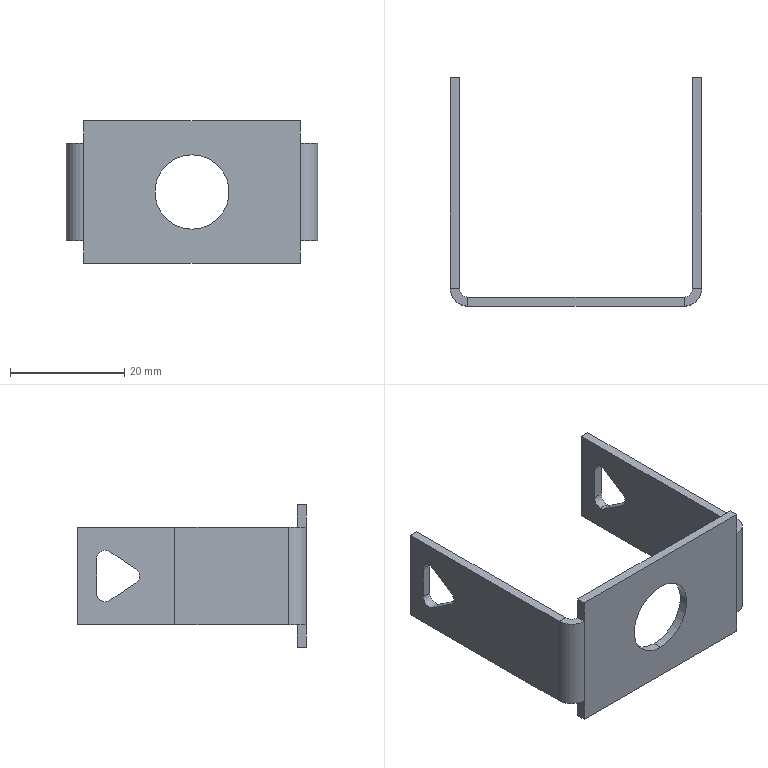Part | SolidWorks | features ICE 6, FlatPattern 1, MirrorPattern 1, SMBaseFlange 1, SheetMetal 1 | 1 solid | 48 faces | box 44 x 40 x 25 mm | volume 3354 mm3 | plane 34 | cylinder 14 | commonest cylinder face diameters 3 x10 6.2 x2 13 x2
STEP:
#1=CARTESIAN_POINT('',(42.401,35.2,-4.497));
#2=VERTEX_POINT('',#1);
#3=CARTESIAN_POINT('',(42.401,36.7,-2.997));
#4=VERTEX_POINT('',#3);
#5=CARTESIAN_POINT('',(42.401,35.2,-2.997));
#6=DIRECTION('',(1.,0.,0.));
#7=DIRECTION('',(0.,0.,-1.));
#8=AXIS2_PLACEMENT_3D('',#5,#6,#7);
#9=CIRCLE('',#8,1.5);
#10=EDGE_CURVE('',#2,#4,#9,.T.);
#11=ORIENTED_EDGE('',*,*,#10,.F.);
#12=CARTESIAN_POINT('',(43.999,35.2,-4.497));
#13=VERTEX_POINT('',#12);
#14=CARTESIAN_POINT('',(40.9,35.2,-4.497));
#15=DIRECTION('',(1.,0.,0.));
#16=VECTOR('',#15,1000.);
#17=LINE('',#14,#16);
#18=EDGE_CURVE('',#2,#13,#17,.T.);
#19=ORIENTED_EDGE('',*,*,#18,.T.);
#20=CARTESIAN_POINT('',(43.999,36.7,-2.997));
#21=VERTEX_POINT('',#20);
#22=CARTESIAN_POINT('',(43.999,35.2,-2.997));
#23=DIRECTION('',(-1.,0.,0.));
#24=DIRECTION('',(0.,0.,1.));
#25=AXIS2_PLACEMENT_3D('',#22,#23,#24);
#26=CIRCLE('',#25,1.5);
#27=EDGE_CURVE('',#21,#13,#26,.T.);
#28=ORIENTED_EDGE('',*,*,#27,.F.);
#29=CARTESIAN_POINT('',(40.9,36.7,-2.997));
#30=DIRECTION('',(1.,0.,0.));
#31=VECTOR('',#30,1000.);
#32=LINE('',#29,#31);
#33=EDGE_CURVE('',#4,#21,#32,.T.);
#34=ORIENTED_EDGE('',*,*,#33,.F.);
#35=EDGE_LOOP('',(#11,#19,#28,#34));
#36=FACE_OUTER_BOUND('',#35,.T.);
#37=CARTESIAN_POINT('',(40.9,35.2,-2.997));
#38=DIRECTION('',(1.,0.,0.));
#39=DIRECTION('',(0.,0.,-1.));
#40=AXIS2_PLACEMENT_3D('',#37,#38,#39);
#41=CYLINDRICAL_SURFACE('',#40,1.5);
#42=ADVANCED_FACE('',(#36),#41,.F.);
#43=CARTESIAN_POINT('',(22.,0.,-6.5));
#44=VERTEX_POINT('',#43);
#45=CARTESIAN_POINT('',(22.,0.,6.5));
#46=VERTEX_POINT('',#45);
#47=CARTESIAN_POINT('',(22.,0.,0.));
#48=DIRECTION('',(0.,1.,0.));
#49=DIRECTION('',(0.,0.,-1.));
#50=AXIS2_PLACEMENT_3D('',#47,#48,#49);
#51=CIRCLE('',#50,6.5);
#52=EDGE_CURVE('',#44,#46,#51,.T.);
#53=ORIENTED_EDGE('',*,*,#52,.F.);
#54=CARTESIAN_POINT('',(22.,1.6,-6.5));
#55=VERTEX_POINT('',#54);
#56=CARTESIAN_POINT('',(22.,-0.001,-6.5));
#57=DIRECTION('',(0.,1.,0.));
#58=VECTOR('',#57,1000.);
#59=LINE('',#56,#58);
#60=EDGE_CURVE('',#44,#55,#59,.T.);
#61=ORIENTED_EDGE('',*,*,#60,.T.);
#62=CARTESIAN_POINT('',(22.,1.6,6.5));
#63=VERTEX_POINT('',#62);
#64=CARTESIAN_POINT('',(22.,1.6,0.));
#65=DIRECTION('',(0.,1.,0.));
#66=DIRECTION('',(0.,0.,1.));
#67=AXIS2_PLACEMENT_3D('',#64,#65,#66);
#68=CIRCLE('',#67,6.5);
#69=EDGE_CURVE('',#55,#63,#68,.T.);
#70=ORIENTED_EDGE('',*,*,#69,.T.);
#71=CARTESIAN_POINT('',(22.,-0.001,6.5));
#72=DIRECTION('',(0.,1.,0.));
#73=VECTOR('',#72,1000.);
#74=LINE('',#71,#73);
#75=EDGE_CURVE('',#46,#63,#74,.T.);
#76=ORIENTED_EDGE('',*,*,#75,.F.);
#77=EDGE_LOOP('',(#53,#61,#70,#76));
#78=FACE_OUTER_BOUND('',#77,.T.);
#79=CARTESIAN_POINT('',(22.,-0.001,0.));
#80=DIRECTION('',(0.,1.,0.));
#81=DIRECTION('',(0.,0.,1.));
#82=AXIS2_PLACEMENT_3D('',#79,#80,#81);
#83=CYLINDRICAL_SURFACE('',#82,6.5);
#84=ADVANCED_FACE('',(#78),#83,.F.);
#85=CARTESIAN_POINT('',(1.599,35.2,4.497));
#86=VERTEX_POINT('',#85);
#87=CARTESIAN_POINT('',(1.599,36.7,2.997));
#88=VERTEX_POINT('',#87);
#89=CARTESIAN_POINT('',(1.599,35.2,2.997));
#90=DIRECTION('',(-1.,0.,0.));
#91=DIRECTION('',(0.,0.,-1.));
#92=AXIS2_PLACEMENT_3D('',#89,#90,#91);
#93=CIRCLE('',#92,1.5);
#94=EDGE_CURVE('',#86,#88,#93,.T.);
#95=ORIENTED_EDGE('',*,*,#94,.F.);
#96=CARTESIAN_POINT('',(0.01,35.2,4.497));
#97=VERTEX_POINT('',#96);
#98=CARTESIAN_POINT('',(3.1,35.2,4.497));
#99=DIRECTION('',(-1.,0.,0.));
#100=VECTOR('',#99,1000.);
#101=LINE('',#98,#100);
#102=EDGE_CURVE('',#86,#97,#101,.T.);
#103=ORIENTED_EDGE('',*,*,#102,.T.);
#104=CARTESIAN_POINT('',(0.01,36.7,2.997));
#105=VERTEX_POINT('',#104);
#106=CARTESIAN_POINT('',(0.01,35.2,2.997));
#107=DIRECTION('',(1.,0.,0.));
#108=DIRECTION('',(0.,0.,1.));
#109=AXIS2_PLACEMENT_3D('',#106,#107,#108);
#110=CIRCLE('',#109,1.5);
#111=EDGE_CURVE('',#105,#97,#110,.T.);
#112=ORIENTED_EDGE('',*,*,#111,.F.);
#113=CARTESIAN_POINT('',(3.1,36.7,2.997));
#114=DIRECTION('',(-1.,0.,0.));
#115=VECTOR('',#114,1000.);
#116=LINE('',#113,#115);
#117=EDGE_CURVE('',#88,#105,#116,.T.);
#118=ORIENTED_EDGE('',*,*,#117,.F.);
#119=EDGE_LOOP('',(#95,#103,#112,#118));
#120=FACE_OUTER_BOUND('',#119,.T.);
#121=CARTESIAN_POINT('',(3.1,35.2,2.997));
#122=DIRECTION('',(-1.,0.,0.));
#123=DIRECTION('',(0.,0.,1.));
#124=AXIS2_PLACEMENT_3D('',#121,#122,#123);
#125=CYLINDRICAL_SURFACE('',#124,1.5);
#126=ADVANCED_FACE('',(#120),#125,.F.);
#127=CARTESIAN_POINT('',(1.599,40.,8.5));
#128=VERTEX_POINT('',#127);
#129=CARTESIAN_POINT('',(0.01,40.,8.5));
#130=VERTEX_POINT('',#129);
#131=CARTESIAN_POINT('',(3.1,40.,8.5));
#132=DIRECTION('',(-1.,0.,0.));
#133=VECTOR('',#132,1000.);
#134=LINE('',#131,#133);
#135=EDGE_CURVE('',#128,#130,#134,.T.);
#136=ORIENTED_EDGE('',*,*,#135,.F.);
#137=CARTESIAN_POINT('',(1.599,40.,-8.5));
#138=VERTEX_POINT('',#137);
#139=CARTESIAN_POINT('',(1.599,40.,8.5));
#140=DIRECTION('',(0.,0.,1.));
#141=VECTOR('',#140,1000.);
#142=LINE('',#139,#141);
#143=EDGE_CURVE('',#138,#128,#142,.T.);
#144=ORIENTED_EDGE('',*,*,#143,.F.);
#145=CARTESIAN_POINT('',(0.01,40.,-8.5));
#146=VERTEX_POINT('',#145);
#147=CARTESIAN_POINT('',(3.1,40.,-8.5));
#148=DIRECTION('',(-1.,0.,0.));
#149=VECTOR('',#148,1000.);
#150=LINE('',#147,#149);
#151=EDGE_CURVE('',#138,#146,#150,.T.);
#152=ORIENTED_EDGE('',*,*,#151,.T.);
#153=CARTESIAN_POINT('',(0.01,40.,-8.5));
#154=DIRECTION('',(0.,0.,-1.));
#155=VECTOR('',#154,1000.);
#156=LINE('',#153,#155);
#157=EDGE_CURVE('',#130,#146,#156,.T.);
#158=ORIENTED_EDGE('',*,*,#157,.F.);
#159=EDGE_LOOP('',(#136,#144,#152,#158));
#160=FACE_OUTER_BOUND('',#159,.T.);
#161=CARTESIAN_POINT('',(0.,40.,12.5));
#162=DIRECTION('',(0.,1.,0.));
#163=DIRECTION('',(0.,0.,1.));
#164=AXIS2_PLACEMENT_3D('',#161,#162,#163);
#165=PLANE('',#164);
#166=ADVANCED_FACE('',(#160),#165,.T.);
#167=CARTESIAN_POINT('',(1.599,29.872,-1.248));
#168=VERTEX_POINT('',#167);
#169=CARTESIAN_POINT('',(1.599,29.872,1.248));
#170=VERTEX_POINT('',#169);
#171=CARTESIAN_POINT('',(1.599,30.704,0.));
#172=DIRECTION('',(-1.,0.,0.));
#173=DIRECTION('',(0.,0.,-1.));
#174=AXIS2_PLACEMENT_3D('',#171,#172,#173);
#175=CIRCLE('',#174,1.5);
#176=EDGE_CURVE('',#168,#170,#175,.T.);
#177=ORIENTED_EDGE('',*,*,#176,.F.);
#178=CARTESIAN_POINT('',(0.01,29.872,-1.248));
#179=VERTEX_POINT('',#178);
#180=CARTESIAN_POINT('',(3.1,29.872,-1.248));
#181=DIRECTION('',(-1.,0.,0.));
#182=VECTOR('',#181,1000.);
#183=LINE('',#180,#182);
#184=EDGE_CURVE('',#168,#179,#183,.T.);
#185=ORIENTED_EDGE('',*,*,#184,.T.);
#186=CARTESIAN_POINT('',(0.01,29.872,1.248));
#187=VERTEX_POINT('',#186);
#188=CARTESIAN_POINT('',(0.01,30.704,0.));
#189=DIRECTION('',(1.,0.,0.));
#190=DIRECTION('',(0.,0.,1.));
#191=AXIS2_PLACEMENT_3D('',#188,#189,#190);
#192=CIRCLE('',#191,1.5);
#193=EDGE_CURVE('',#187,#179,#192,.T.);
#194=ORIENTED_EDGE('',*,*,#193,.F.);
#195=CARTESIAN_POINT('',(3.1,29.872,1.248));
#196=DIRECTION('',(-1.,0.,0.));
#197=VECTOR('',#196,1000.);
#198=LINE('',#195,#197);
#199=EDGE_CURVE('',#170,#187,#198,.T.);
#200=ORIENTED_EDGE('',*,*,#199,.F.);
#201=EDGE_LOOP('',(#177,#185,#194,#200));
#202=FACE_OUTER_BOUND('',#201,.T.);
#203=CARTESIAN_POINT('',(3.1,30.704,0.));
#204=DIRECTION('',(-1.,0.,0.));
#205=DIRECTION('',(0.,0.,1.));
#206=AXIS2_PLACEMENT_3D('',#203,#204,#205);
#207=CYLINDRICAL_SURFACE('',#206,1.5);
#208=ADVANCED_FACE('',(#202),#207,.F.);
#209=CARTESIAN_POINT('',(1.599,34.368,-4.245));
#210=VERTEX_POINT('',#209);
#211=CARTESIAN_POINT('',(1.599,29.872,-1.248));
#212=DIRECTION('',(0.,-0.8321,0.5547));
#213=VECTOR('',#212,1000.);
#214=LINE('',#211,#213);
#215=EDGE_CURVE('',#210,#168,#214,.T.);
#216=ORIENTED_EDGE('',*,*,#215,.F.);
#217=CARTESIAN_POINT('',(0.01,34.368,-4.245));
#218=VERTEX_POINT('',#217);
#219=CARTESIAN_POINT('',(3.1,34.368,-4.245));
#220=DIRECTION('',(-1.,0.,0.));
#221=VECTOR('',#220,1000.);
#222=LINE('',#219,#221);
#223=EDGE_CURVE('',#210,#218,#222,.T.);
#224=ORIENTED_EDGE('',*,*,#223,.T.);
#225=CARTESIAN_POINT('',(0.01,29.872,-1.248));
#226=DIRECTION('',(0.,0.8321,-0.5547));
#227=VECTOR('',#226,1000.);
#228=LINE('',#225,#227);
#229=EDGE_CURVE('',#179,#218,#228,.T.);
#230=ORIENTED_EDGE('',*,*,#229,.F.);
#231=ORIENTED_EDGE('',*,*,#184,.F.);
#232=EDGE_LOOP('',(#216,#224,#230,#231));
#233=FACE_OUTER_BOUND('',#232,.T.);
#234=CARTESIAN_POINT('',(3.1,29.872,-1.248));
#235=DIRECTION('',(0.,-0.5547,-0.8321));
#236=DIRECTION('',(0.,0.8321,-0.5547));
#237=AXIS2_PLACEMENT_3D('',#234,#235,#236);
#238=PLANE('',#237);
#239=ADVANCED_FACE('',(#233),#238,.F.);
#240=CARTESIAN_POINT('',(1.599,36.7,-2.997));
#241=VERTEX_POINT('',#240);
#242=CARTESIAN_POINT('',(1.599,35.2,-2.997));
#243=DIRECTION('',(-1.,0.,0.));
#244=DIRECTION('',(0.,0.,-1.));
#245=AXIS2_PLACEMENT_3D('',#242,#243,#244);
#246=CIRCLE('',#245,1.5);
#247=EDGE_CURVE('',#241,#210,#246,.T.);
#248=ORIENTED_EDGE('',*,*,#247,.F.);
#249=CARTESIAN_POINT('',(0.01,36.7,-2.997));
#250=VERTEX_POINT('',#249);
#251=CARTESIAN_POINT('',(3.1,36.7,-2.997));
#252=DIRECTION('',(-1.,0.,0.));
#253=VECTOR('',#252,1000.);
#254=LINE('',#251,#253);
#255=EDGE_CURVE('',#241,#250,#254,.T.);
#256=ORIENTED_EDGE('',*,*,#255,.T.);
#257=CARTESIAN_POINT('',(0.01,35.2,-2.997));
#258=DIRECTION('',(1.,0.,0.));
#259=DIRECTION('',(0.,0.,1.));
#260=AXIS2_PLACEMENT_3D('',#257,#258,#259);
#261=CIRCLE('',#260,1.5);
#262=EDGE_CURVE('',#218,#250,#261,.T.);
#263=ORIENTED_EDGE('',*,*,#262,.F.);
#264=ORIENTED_EDGE('',*,*,#223,.F.);
#265=EDGE_LOOP('',(#248,#256,#263,#264));
#266=FACE_OUTER_BOUND('',#265,.T.);
#267=CARTESIAN_POINT('',(3.1,35.2,-2.997));
#268=DIRECTION('',(-1.,0.,0.));
#269=DIRECTION('',(0.,0.,1.));
#270=AXIS2_PLACEMENT_3D('',#267,#268,#269);
#271=CYLINDRICAL_SURFACE('',#270,1.5);
#272=ADVANCED_FACE('',(#266),#271,.F.);
#273=CARTESIAN_POINT('',(1.599,36.7,-2.997));
#274=DIRECTION('',(0.,0.,-1.));
#275=VECTOR('',#274,1000.);
#276=LINE('',#273,#275);
#277=EDGE_CURVE('',#88,#241,#276,.T.);
#278=ORIENTED_EDGE('',*,*,#277,.F.);
#279=ORIENTED_EDGE('',*,*,#117,.T.);
#280=CARTESIAN_POINT('',(0.01,36.7,-2.997));
#281=DIRECTION('',(0.,0.,1.));
#282=VECTOR('',#281,1000.);
#283=LINE('',#280,#282);
#284=EDGE_CURVE('',#250,#105,#283,.T.);
#285=ORIENTED_EDGE('',*,*,#284,.F.);
#286=ORIENTED_EDGE('',*,*,#255,.F.);
#287=EDGE_LOOP('',(#278,#279,#285,#286));
#288=FACE_OUTER_BOUND('',#287,.T.);
#289=CARTESIAN_POINT('',(3.1,36.7,-2.997));
#290=DIRECTION('',(0.,1.,0.));
#291=DIRECTION('',(0.,0.,1.));
#292=AXIS2_PLACEMENT_3D('',#289,#290,#291);
#293=PLANE('',#292);
#294=ADVANCED_FACE('',(#288),#293,.F.);
#295=ORIENTED_EDGE('',*,*,#102,.F.);
#296=CARTESIAN_POINT('',(1.599,34.368,4.245));
#297=VERTEX_POINT('',#296);
#298=CARTESIAN_POINT('',(1.599,35.2,2.997));
#299=DIRECTION('',(-1.,0.,0.));
#300=DIRECTION('',(0.,0.,-1.));
#301=AXIS2_PLACEMENT_3D('',#298,#299,#300);
#302=CIRCLE('',#301,1.5);
#303=EDGE_CURVE('',#297,#86,#302,.T.);
#304=ORIENTED_EDGE('',*,*,#303,.F.);
#305=CARTESIAN_POINT('',(0.01,34.368,4.245));
#306=VERTEX_POINT('',#305);
#307=CARTESIAN_POINT('',(3.1,34.368,4.245));
#308=DIRECTION('',(-1.,0.,0.));
#309=VECTOR('',#308,1000.);
#310=LINE('',#307,#309);
#311=EDGE_CURVE('',#297,#306,#310,.T.);
#312=ORIENTED_EDGE('',*,*,#311,.T.);
#313=CARTESIAN_POINT('',(0.01,35.2,2.997));
#314=DIRECTION('',(1.,0.,0.));
#315=DIRECTION('',(0.,0.,1.));
#316=AXIS2_PLACEMENT_3D('',#313,#314,#315);
#317=CIRCLE('',#316,1.5);
#318=EDGE_CURVE('',#97,#306,#317,.T.);
#319=ORIENTED_EDGE('',*,*,#318,.F.);
#320=EDGE_LOOP('',(#295,#304,#312,#319));
#321=FACE_OUTER_BOUND('',#320,.T.);
#322=CARTESIAN_POINT('',(3.1,35.2,2.997));
#323=DIRECTION('',(-1.,0.,0.));
#324=DIRECTION('',(0.,0.,1.));
#325=AXIS2_PLACEMENT_3D('',#322,#323,#324);
#326=CYLINDRICAL_SURFACE('',#325,1.5);
#327=ADVANCED_FACE('',(#321),#326,.F.);
#328=CARTESIAN_POINT('',(1.599,29.872,1.248));
#329=DIRECTION('',(0.,0.8321,0.5547));
#330=VECTOR('',#329,1000.);
#331=LINE('',#328,#330);
#332=EDGE_CURVE('',#170,#297,#331,.T.);
#333=ORIENTED_EDGE('',*,*,#332,.F.);
#334=ORIENTED_EDGE('',*,*,#199,.T.);
#335=CARTESIAN_POINT('',(0.01,29.872,1.248));
#336=DIRECTION('',(0.,-0.8321,-0.5547));
#337=VECTOR('',#336,1000.);
#338=LINE('',#335,#337);
#339=EDGE_CURVE('',#306,#187,#338,.T.);
#340=ORIENTED_EDGE('',*,*,#339,.F.);
#341=ORIENTED_EDGE('',*,*,#311,.F.);
#342=EDGE_LOOP('',(#333,#334,#340,#341));
#343=FACE_OUTER_BOUND('',#342,.T.);
#344=CARTESIAN_POINT('',(3.1,29.872,1.248));
#345=DIRECTION('',(0.,-0.5547,0.8321));
#346=DIRECTION('',(0.,-0.8321,-0.5547));
#347=AXIS2_PLACEMENT_3D('',#344,#345,#346);
#348=PLANE('',#347);
#349=ADVANCED_FACE('',(#343),#348,.F.);
#350=CARTESIAN_POINT('',(42.401,23.,8.5));
#351=VERTEX_POINT('',#350);
#352=CARTESIAN_POINT('',(42.4,23.,8.5));
#353=VERTEX_POINT('',#352);
#354=CARTESIAN_POINT('',(42.401,23.,8.5));
#355=DIRECTION('',(-1.,0.,0.));
#356=VECTOR('',#355,1000.);
#357=LINE('',#354,#356);
#358=EDGE_CURVE('',#351,#353,#357,.T.);
#359=ORIENTED_EDGE('',*,*,#358,.T.);
#360=CARTESIAN_POINT('',(42.4,3.1,8.5));
#361=VERTEX_POINT('',#360);
#362=CARTESIAN_POINT('',(42.4,0.,8.5));
#363=DIRECTION('',(0.,-1.,0.));
#364=VECTOR('',#363,1000.);
#365=LINE('',#362,#364);
#366=EDGE_CURVE('',#353,#361,#365,.T.);
#367=ORIENTED_EDGE('',*,*,#366,.T.);
#368=CARTESIAN_POINT('',(44.,3.1,8.5));
#369=VERTEX_POINT('',#368);
#370=CARTESIAN_POINT('',(42.4,3.1,8.5));
#371=DIRECTION('',(1.,0.,0.));
#372=VECTOR('',#371,1000.);
#373=LINE('',#370,#372);
#374=EDGE_CURVE('',#361,#369,#373,.T.);
#375=ORIENTED_EDGE('',*,*,#374,.T.);
#376=CARTESIAN_POINT('',(44.,23.,8.5));
#377=VERTEX_POINT('',#376);
#378=CARTESIAN_POINT('',(44.,40.,8.5));
#379=DIRECTION('',(0.,-1.,0.));
#380=VECTOR('',#379,1000.);
#381=LINE('',#378,#380);
#382=EDGE_CURVE('',#377,#369,#381,.T.);
#383=ORIENTED_EDGE('',*,*,#382,.F.);
#384=CARTESIAN_POINT('',(43.999,23.,8.5));
#385=VERTEX_POINT('',#384);
#386=CARTESIAN_POINT('',(43.999,23.,8.5));
#387=DIRECTION('',(1.,0.,0.));
#388=VECTOR('',#387,1000.);
#389=LINE('',#386,#388);
#390=EDGE_CURVE('',#385,#377,#389,.T.);
#391=ORIENTED_EDGE('',*,*,#390,.F.);
#392=CARTESIAN_POINT('',(43.999,40.,8.5));
#393=VERTEX_POINT('',#392);
#394=CARTESIAN_POINT('',(43.999,40.,8.5));
#395=DIRECTION('',(0.,-1.,0.));
#396=VECTOR('',#395,1000.);
#397=LINE('',#394,#396);
#398=EDGE_CURVE('',#393,#385,#397,.T.);
#399=ORIENTED_EDGE('',*,*,#398,.F.);
#400=CARTESIAN_POINT('',(42.401,40.,8.5));
#401=VERTEX_POINT('',#400);
#402=CARTESIAN_POINT('',(40.9,40.,8.5));
#403=DIRECTION('',(1.,0.,0.));
#404=VECTOR('',#403,1000.);
#405=LINE('',#402,#404);
#406=EDGE_CURVE('',#401,#393,#405,.T.);
#407=ORIENTED_EDGE('',*,*,#406,.F.);
#408=CARTESIAN_POINT('',(42.401,40.,8.5));
#409=DIRECTION('',(0.,1.,0.));
#410=VECTOR('',#409,1000.);
#411=LINE('',#408,#410);
#412=EDGE_CURVE('',#351,#401,#411,.T.);
#413=ORIENTED_EDGE('',*,*,#412,.F.);
#414=EDGE_LOOP('',(#359,#367,#375,#383,#391,#399,#407,#413));
#415=FACE_OUTER_BOUND('',#414,.T.);
#416=CARTESIAN_POINT('',(40.9,40.,8.5));
#417=DIRECTION('',(0.,0.,1.));
#418=DIRECTION('',(0.,-1.,0.));
#419=AXIS2_PLACEMENT_3D('',#416,#417,#418);
#420=PLANE('',#419);
#421=ADVANCED_FACE('',(#415),#420,.T.);
#422=CARTESIAN_POINT('',(40.9,0.,8.5));
#423=VERTEX_POINT('',#422);
#424=CARTESIAN_POINT('',(40.9,0.,-8.5));
#425=VERTEX_POINT('',#424);
#426=CARTESIAN_POINT('',(40.9,0.,12.5));
#427=DIRECTION('',(0.,0.,-1.));
#428=VECTOR('',#427,1000.);
#429=LINE('',#426,#428);
#430=EDGE_CURVE('',#423,#425,#429,.T.);
#431=ORIENTED_EDGE('',*,*,#430,.T.);
#432=CARTESIAN_POINT('',(44.,3.1,-8.5));
#433=VERTEX_POINT('',#432);
#434=CARTESIAN_POINT('',(40.9,3.1,-8.5));
#435=DIRECTION('',(0.,0.,1.));
#436=DIRECTION('',(0.,1.,0.));
#437=AXIS2_PLACEMENT_3D('',#434,#435,#436);
#438=CIRCLE('',#437,3.1);
#439=EDGE_CURVE('',#425,#433,#438,.T.);
#440=ORIENTED_EDGE('',*,*,#439,.T.);
#441=CARTESIAN_POINT('',(44.,3.1,12.5));
#442=DIRECTION('',(0.,0.,-1.));
#443=VECTOR('',#442,1000.);
#444=LINE('',#441,#443);
#445=EDGE_CURVE('',#369,#433,#444,.T.);
#446=ORIENTED_EDGE('',*,*,#445,.F.);
#447=CARTESIAN_POINT('',(40.9,3.1,8.5));
#448=DIRECTION('',(0.,0.,-1.));
#449=DIRECTION('',(0.,-1.,0.));
#450=AXIS2_PLACEMENT_3D('',#447,#448,#449);
#451=CIRCLE('',#450,3.1);
#452=EDGE_CURVE('',#369,#423,#451,.T.);
#453=ORIENTED_EDGE('',*,*,#452,.T.);
#454=EDGE_LOOP('',(#431,#440,#446,#453));
#455=FACE_OUTER_BOUND('',#454,.T.);
#456=CARTESIAN_POINT('',(40.9,3.1,12.5));
#457=DIRECTION('',(0.,0.,-1.));
#458=DIRECTION('',(-1.,0.,0.));
#459=AXIS2_PLACEMENT_3D('',#456,#457,#458);
#460=CYLINDRICAL_SURFACE('',#459,3.1);
#461=ADVANCED_FACE('',(#455),#460,.T.);
#462=CARTESIAN_POINT('',(44.,23.,-8.5));
#463=VERTEX_POINT('',#462);
#464=CARTESIAN_POINT('',(44.,23.,-8.5));
#465=DIRECTION('',(0.,0.,-1.));
#466=VECTOR('',#465,1000.);
#467=LINE('',#464,#466);
#468=EDGE_CURVE('',#377,#463,#467,.T.);
#469=ORIENTED_EDGE('',*,*,#468,.F.);
#470=ORIENTED_EDGE('',*,*,#382,.T.);
#471=ORIENTED_EDGE('',*,*,#445,.T.);
#472=CARTESIAN_POINT('',(44.,40.,-8.5));
#473=DIRECTION('',(0.,1.,0.));
#474=VECTOR('',#473,1000.);
#475=LINE('',#472,#474);
#476=EDGE_CURVE('',#433,#463,#475,.T.);
#477=ORIENTED_EDGE('',*,*,#476,.T.);
#478=EDGE_LOOP('',(#469,#470,#471,#477));
#479=FACE_OUTER_BOUND('',#478,.T.);
#480=CARTESIAN_POINT('',(44.,0.,12.5));
#481=DIRECTION('',(1.,0.,0.));
#482=DIRECTION('',(0.,0.,-1.));
#483=AXIS2_PLACEMENT_3D('',#480,#481,#482);
#484=PLANE('',#483);
#485=ADVANCED_FACE('',(#479),#484,.T.);
#486=CARTESIAN_POINT('',(42.401,40.,-8.5));
#487=VERTEX_POINT('',#486);
#488=CARTESIAN_POINT('',(42.401,40.,8.5));
#489=DIRECTION('',(0.,0.,-1.));
#490=VECTOR('',#489,1000.);
#491=LINE('',#488,#490);
#492=EDGE_CURVE('',#401,#487,#491,.T.);
#493=ORIENTED_EDGE('',*,*,#492,.F.);
#494=ORIENTED_EDGE('',*,*,#406,.T.);
#495=CARTESIAN_POINT('',(43.999,40.,-8.5));
#496=VERTEX_POINT('',#495);
#497=CARTESIAN_POINT('',(43.999,40.,-8.5));
#498=DIRECTION('',(0.,0.,1.));
#499=VECTOR('',#498,1000.);
#500=LINE('',#497,#499);
#501=EDGE_CURVE('',#496,#393,#500,.T.);
#502=ORIENTED_EDGE('',*,*,#501,.F.);
#503=CARTESIAN_POINT('',(40.9,40.,-8.5));
#504=DIRECTION('',(1.,0.,0.));
#505=VECTOR('',#504,1000.);
#506=LINE('',#503,#505);
#507=EDGE_CURVE('',#487,#496,#506,.T.);
#508=ORIENTED_EDGE('',*,*,#507,.F.);
#509=EDGE_LOOP('',(#493,#494,#502,#508));
#510=FACE_OUTER_BOUND('',#509,.T.);
#511=CARTESIAN_POINT('',(42.4,40.,12.5));
#512=DIRECTION('',(0.,1.,0.));
#513=DIRECTION('',(0.,0.,1.));
#514=AXIS2_PLACEMENT_3D('',#511,#512,#513);
#515=PLANE('',#514);
#516=ADVANCED_FACE('',(#510),#515,.T.);
#517=ORIENTED_EDGE('',*,*,#366,.F.);
#518=CARTESIAN_POINT('',(42.4,23.,-8.5));
#519=VERTEX_POINT('',#518);
#520=CARTESIAN_POINT('',(42.4,23.,8.5));
#521=DIRECTION('',(0.,0.,1.));
#522=VECTOR('',#521,1000.);
#523=LINE('',#520,#522);
#524=EDGE_CURVE('',#519,#353,#523,.T.);
#525=ORIENTED_EDGE('',*,*,#524,.F.);
#526=CARTESIAN_POINT('',(42.4,3.1,-8.5));
#527=VERTEX_POINT('',#526);
#528=CARTESIAN_POINT('',(42.4,0.,-8.5));
#529=DIRECTION('',(0.,1.,0.));
#530=VECTOR('',#529,1000.);
#531=LINE('',#528,#530);
#532=EDGE_CURVE('',#527,#519,#531,.T.);
#533=ORIENTED_EDGE('',*,*,#532,.F.);
#534=CARTESIAN_POINT('',(42.4,3.1,12.5));
#535=DIRECTION('',(0.,0.,-1.));
#536=VECTOR('',#535,1000.);
#537=LINE('',#534,#536);
#538=EDGE_CURVE('',#361,#527,#537,.T.);
#539=ORIENTED_EDGE('',*,*,#538,.F.);
#540=EDGE_LOOP('',(#517,#525,#533,#539));
#541=FACE_OUTER_BOUND('',#540,.T.);
#542=CARTESIAN_POINT('',(42.4,0.,12.5));
#543=DIRECTION('',(1.,0.,0.));
#544=DIRECTION('',(0.,0.,-1.));
#545=AXIS2_PLACEMENT_3D('',#542,#543,#544);
#546=PLANE('',#545);
#547=ADVANCED_FACE('',(#541),#546,.F.);
#548=CARTESIAN_POINT('',(40.9,1.6,-8.5));
#549=VERTEX_POINT('',#548);
#550=CARTESIAN_POINT('',(40.9,3.1,-8.5));
#551=DIRECTION('',(0.,0.,1.));
#552=DIRECTION('',(0.,1.,0.));
#553=AXIS2_PLACEMENT_3D('',#550,#551,#552);
#554=CIRCLE('',#553,1.5);
#555=EDGE_CURVE('',#549,#527,#554,.T.);
#556=ORIENTED_EDGE('',*,*,#555,.F.);
#557=CARTESIAN_POINT('',(40.9,1.6,8.5));
#558=VERTEX_POINT('',#557);
#559=CARTESIAN_POINT('',(40.9,1.6,12.5));
#560=DIRECTION('',(0.,0.,-1.));
#561=VECTOR('',#560,1000.);
#562=LINE('',#559,#561);
#563=EDGE_CURVE('',#558,#549,#562,.T.);
#564=ORIENTED_EDGE('',*,*,#563,.F.);
#565=CARTESIAN_POINT('',(40.9,3.1,8.5));
#566=DIRECTION('',(0.,0.,-1.));
#567=DIRECTION('',(0.,-1.,0.));
#568=AXIS2_PLACEMENT_3D('',#565,#566,#567);
#569=CIRCLE('',#568,1.5);
#570=EDGE_CURVE('',#361,#558,#569,.T.);
#571=ORIENTED_EDGE('',*,*,#570,.F.);
#572=ORIENTED_EDGE('',*,*,#538,.T.);
#573=EDGE_LOOP('',(#556,#564,#571,#572));
#574=FACE_OUTER_BOUND('',#573,.T.);
#575=CARTESIAN_POINT('',(40.9,3.1,12.5));
#576=DIRECTION('',(0.,0.,-1.));
#577=DIRECTION('',(-1.,0.,0.));
#578=AXIS2_PLACEMENT_3D('',#575,#576,#577);
#579=CYLINDRICAL_SURFACE('',#578,1.5);
#580=ADVANCED_FACE('',(#574),#579,.F.);
#581=CARTESIAN_POINT('',(1.6,23.,8.5));
#582=VERTEX_POINT('',#581);
#583=CARTESIAN_POINT('',(1.6,3.1,8.5));
#584=VERTEX_POINT('',#583);
#585=CARTESIAN_POINT('',(1.6,0.,8.5));
#586=DIRECTION('',(0.,-1.,0.));
#587=VECTOR('',#586,1000.);
#588=LINE('',#585,#587);
#589=EDGE_CURVE('',#582,#584,#588,.T.);
#590=ORIENTED_EDGE('',*,*,#589,.F.);
#591=CARTESIAN_POINT('',(1.599,23.,8.5));
#592=VERTEX_POINT('',#591);
#593=CARTESIAN_POINT('',(1.599,23.,8.5));
#594=DIRECTION('',(1.,0.,0.));
#595=VECTOR('',#594,1000.);
#596=LINE('',#593,#595);
#597=EDGE_CURVE('',#592,#582,#596,.T.);
#598=ORIENTED_EDGE('',*,*,#597,.F.);
#599=CARTESIAN_POINT('',(1.599,40.,8.5));
#600=DIRECTION('',(0.,-1.,0.));
#601=VECTOR('',#600,1000.);
#602=LINE('',#599,#601);
#603=EDGE_CURVE('',#128,#592,#602,.T.);
#604=ORIENTED_EDGE('',*,*,#603,.F.);
#605=ORIENTED_EDGE('',*,*,#135,.T.);
#606=CARTESIAN_POINT('',(0.01,23.,8.5));
#607=VERTEX_POINT('',#606);
#608=CARTESIAN_POINT('',(0.01,40.,8.5));
#609=DIRECTION('',(0.,1.,0.));
#610=VECTOR('',#609,1000.);
#611=LINE('',#608,#610);
#612=EDGE_CURVE('',#607,#130,#611,.T.);
#613=ORIENTED_EDGE('',*,*,#612,.F.);
#614=CARTESIAN_POINT('',(0.,23.,8.5));
#615=VERTEX_POINT('',#614);
#616=CARTESIAN_POINT('',(0.01,23.,8.5));
#617=DIRECTION('',(-1.,0.,0.));
#618=VECTOR('',#617,1000.);
#619=LINE('',#616,#618);
#620=EDGE_CURVE('',#607,#615,#619,.T.);
#621=ORIENTED_EDGE('',*,*,#620,.T.);
#622=CARTESIAN_POINT('',(0.,3.1,8.5));
#623=VERTEX_POINT('',#622);
#624=CARTESIAN_POINT('',(0.,40.,8.5));
#625=DIRECTION('',(0.,-1.,0.));
#626=VECTOR('',#625,1000.);
#627=LINE('',#624,#626);
#628=EDGE_CURVE('',#615,#623,#627,.T.);
#629=ORIENTED_EDGE('',*,*,#628,.T.);
#630=CARTESIAN_POINT('',(0.,3.1,8.5));
#631=DIRECTION('',(1.,0.,0.));
#632=VECTOR('',#631,1000.);
#633=LINE('',#630,#632);
#634=EDGE_CURVE('',#623,#584,#633,.T.);
#635=ORIENTED_EDGE('',*,*,#634,.T.);
#636=EDGE_LOOP('',(#590,#598,#604,#605,#613,#621,#629,#635));
#637=FACE_OUTER_BOUND('',#636,.T.);
#638=CARTESIAN_POINT('',(3.1,40.,8.5));
#639=DIRECTION('',(0.,0.,-1.));
#640=DIRECTION('',(0.,1.,0.));
#641=AXIS2_PLACEMENT_3D('',#638,#639,#640);
#642=PLANE('',#641);
#643=ADVANCED_FACE('',(#637),#642,.F.);
#644=CARTESIAN_POINT('',(40.9,0.,-12.5));
#645=VERTEX_POINT('',#644);
#646=CARTESIAN_POINT('',(3.1,0.,-12.5));
#647=VERTEX_POINT('',#646);
#648=CARTESIAN_POINT('',(0.,0.,-12.5));
#649=DIRECTION('',(-1.,0.,0.));
#650=VECTOR('',#649,1000.);
#651=LINE('',#648,#650);
#652=EDGE_CURVE('',#645,#647,#651,.T.);
#653=ORIENTED_EDGE('',*,*,#652,.T.);
#654=CARTESIAN_POINT('',(3.1,1.6,-12.5));
#655=VERTEX_POINT('',#654);
#656=CARTESIAN_POINT('',(3.1,0.,-12.5));
#657=DIRECTION('',(0.,1.,0.));
#658=VECTOR('',#657,1000.);
#659=LINE('',#656,#658);
#660=EDGE_CURVE('',#647,#655,#659,.T.);
#661=ORIENTED_EDGE('',*,*,#660,.T.);
#662=CARTESIAN_POINT('',(40.9,1.6,-12.5));
#663=VERTEX_POINT('',#662);
#664=CARTESIAN_POINT('',(0.,1.6,-12.5));
#665=DIRECTION('',(-1.,0.,0.));
#666=VECTOR('',#665,1000.);
#667=LINE('',#664,#666);
#668=EDGE_CURVE('',#663,#655,#667,.T.);
#669=ORIENTED_EDGE('',*,*,#668,.F.);
#670=CARTESIAN_POINT('',(40.9,1.6,-12.5));
#671=DIRECTION('',(0.,-1.,0.));
#672=VECTOR('',#671,1000.);
#673=LINE('',#670,#672);
#674=EDGE_CURVE('',#663,#645,#673,.T.);
#675=ORIENTED_EDGE('',*,*,#674,.T.);
#676=EDGE_LOOP('',(#653,#661,#669,#675));
#677=FACE_OUTER_BOUND('',#676,.T.);
#678=CARTESIAN_POINT('',(1.6,3.1,-12.5));
#679=DIRECTION('',(0.,0.,-1.));
#680=DIRECTION('',(-1.,0.,0.));
#681=AXIS2_PLACEMENT_3D('',#678,#679,#680);
#682=PLANE('',#681);
#683=ADVANCED_FACE('',(#677),#682,.T.);
#684=CARTESIAN_POINT('',(40.9,0.,12.5));
#685=VERTEX_POINT('',#684);
#686=CARTESIAN_POINT('',(3.1,0.,12.5));
#687=VERTEX_POINT('',#686);
#688=CARTESIAN_POINT('',(0.,0.,12.5));
#689=DIRECTION('',(-1.,0.,0.));
#690=VECTOR('',#689,1000.);
#691=LINE('',#688,#690);
#692=EDGE_CURVE('',#685,#687,#691,.T.);
#693=ORIENTED_EDGE('',*,*,#692,.F.);
#694=CARTESIAN_POINT('',(40.9,1.6,12.5));
#695=VERTEX_POINT('',#694);
#696=CARTESIAN_POINT('',(40.9,0.,12.5));
#697=DIRECTION('',(0.,1.,0.));
#698=VECTOR('',#697,1000.);
#699=LINE('',#696,#698);
#700=EDGE_CURVE('',#685,#695,#699,.T.);
#701=ORIENTED_EDGE('',*,*,#700,.T.);
#702=CARTESIAN_POINT('',(3.1,1.6,12.5));
#703=VERTEX_POINT('',#702);
#704=CARTESIAN_POINT('',(0.,1.6,12.5));
#705=DIRECTION('',(-1.,0.,0.));
#706=VECTOR('',#705,1000.);
#707=LINE('',#704,#706);
#708=EDGE_CURVE('',#695,#703,#707,.T.);
#709=ORIENTED_EDGE('',*,*,#708,.T.);
#710=CARTESIAN_POINT('',(3.1,1.6,12.5));
#711=DIRECTION('',(0.,-1.,0.));
#712=VECTOR('',#711,1000.);
#713=LINE('',#710,#712);
#714=EDGE_CURVE('',#703,#687,#713,.T.);
#715=ORIENTED_EDGE('',*,*,#714,.T.);
#716=EDGE_LOOP('',(#693,#701,#709,#715));
#717=FACE_OUTER_BOUND('',#716,.T.);
#718=CARTESIAN_POINT('',(42.4,3.1,12.5));
#719=DIRECTION('',(0.,0.,1.));
#720=DIRECTION('',(1.,0.,0.));
#721=AXIS2_PLACEMENT_3D('',#718,#719,#720);
#722=PLANE('',#721);
#723=ADVANCED_FACE('',(#717),#722,.T.);
#724=CARTESIAN_POINT('',(1.6,3.1,-8.5));
#725=VERTEX_POINT('',#724);
#726=CARTESIAN_POINT('',(1.6,23.,-8.5));
#727=VERTEX_POINT('',#726);
#728=CARTESIAN_POINT('',(1.6,0.,-8.5));
#729=DIRECTION('',(0.,1.,0.));
#730=VECTOR('',#729,1000.);
#731=LINE('',#728,#730);
#732=EDGE_CURVE('',#725,#727,#731,.T.);
#733=ORIENTED_EDGE('',*,*,#732,.T.);
#734=CARTESIAN_POINT('',(1.6,23.,8.5));
#735=DIRECTION('',(0.,0.,-1.));
#736=VECTOR('',#735,1000.);
#737=LINE('',#734,#736);
#738=EDGE_CURVE('',#582,#727,#737,.T.);
#739=ORIENTED_EDGE('',*,*,#738,.F.);
#740=ORIENTED_EDGE('',*,*,#589,.T.);
#741=CARTESIAN_POINT('',(1.6,3.1,12.5));
#742=DIRECTION('',(0.,0.,-1.));
#743=VECTOR('',#742,1000.);
#744=LINE('',#741,#743);
#745=EDGE_CURVE('',#584,#725,#744,.T.);
#746=ORIENTED_EDGE('',*,*,#745,.T.);
#747=EDGE_LOOP('',(#733,#739,#740,#746));
#748=FACE_OUTER_BOUND('',#747,.T.);
#749=CARTESIAN_POINT('',(1.6,0.,12.5));
#750=DIRECTION('',(-1.,0.,0.));
#751=DIRECTION('',(0.,0.,1.));
#752=AXIS2_PLACEMENT_3D('',#749,#750,#751);
#753=PLANE('',#752);
#754=ADVANCED_FACE('',(#748),#753,.F.);
#755=CARTESIAN_POINT('',(0.,23.,-8.5));
#756=VERTEX_POINT('',#755);
#757=CARTESIAN_POINT('',(0.,23.,-8.5));
#758=DIRECTION('',(0.,0.,1.));
#759=VECTOR('',#758,1000.);
#760=LINE('',#757,#759);
#761=EDGE_CURVE('',#756,#615,#760,.T.);
#762=ORIENTED_EDGE('',*,*,#761,.F.);
#763=CARTESIAN_POINT('',(0.,3.1,-8.5));
#764=VERTEX_POINT('',#763);
#765=CARTESIAN_POINT('',(0.,40.,-8.5));
#766=DIRECTION('',(0.,1.,0.));
#767=VECTOR('',#766,1000.);
#768=LINE('',#765,#767);
#769=EDGE_CURVE('',#764,#756,#768,.T.);
#770=ORIENTED_EDGE('',*,*,#769,.F.);
#771=CARTESIAN_POINT('',(0.,3.1,12.5));
#772=DIRECTION('',(0.,0.,-1.));
#773=VECTOR('',#772,1000.);
#774=LINE('',#771,#773);
#775=EDGE_CURVE('',#623,#764,#774,.T.);
#776=ORIENTED_EDGE('',*,*,#775,.F.);
#777=ORIENTED_EDGE('',*,*,#628,.F.);
#778=EDGE_LOOP('',(#762,#770,#776,#777));
#779=FACE_OUTER_BOUND('',#778,.T.);
#780=CARTESIAN_POINT('',(0.,0.,12.5));
#781=DIRECTION('',(-1.,0.,0.));
#782=DIRECTION('',(0.,0.,1.));
#783=AXIS2_PLACEMENT_3D('',#780,#781,#782);
#784=PLANE('',#783);
#785=ADVANCED_FACE('',(#779),#784,.T.);
#786=CARTESIAN_POINT('',(3.1,0.,-8.5));
#787=VERTEX_POINT('',#786);
#788=CARTESIAN_POINT('',(3.1,3.1,-8.5));
#789=DIRECTION('',(0.,0.,-1.));
#790=DIRECTION('',(0.,-1.,0.));
#791=AXIS2_PLACEMENT_3D('',#788,#789,#790);
#792=CIRCLE('',#791,3.1);
#793=EDGE_CURVE('',#787,#764,#792,.T.);
#794=ORIENTED_EDGE('',*,*,#793,.F.);
#795=CARTESIAN_POINT('',(3.1,0.,8.5));
#796=VERTEX_POINT('',#795);
#797=CARTESIAN_POINT('',(3.1,0.,12.5));
#798=DIRECTION('',(0.,0.,-1.));
#799=VECTOR('',#798,1000.);
#800=LINE('',#797,#799);
#801=EDGE_CURVE('',#796,#787,#800,.T.);
#802=ORIENTED_EDGE('',*,*,#801,.F.);
#803=CARTESIAN_POINT('',(3.1,3.1,8.5));
#804=DIRECTION('',(0.,0.,1.));
#805=DIRECTION('',(0.,1.,0.));
#806=AXIS2_PLACEMENT_3D('',#803,#804,#805);
#807=CIRCLE('',#806,3.1);
#808=EDGE_CURVE('',#623,#796,#807,.T.);
#809=ORIENTED_EDGE('',*,*,#808,.F.);
#810=ORIENTED_EDGE('',*,*,#775,.T.);
#811=EDGE_LOOP('',(#794,#802,#809,#810));
#812=FACE_OUTER_BOUND('',#811,.T.);
#813=CARTESIAN_POINT('',(3.1,3.1,12.5));
#814=DIRECTION('',(0.,0.,-1.));
#815=DIRECTION('',(-1.,0.,0.));
#816=AXIS2_PLACEMENT_3D('',#813,#814,#815);
#817=CYLINDRICAL_SURFACE('',#816,3.1);
#818=ADVANCED_FACE('',(#812),#817,.T.);
#819=CARTESIAN_POINT('',(22.,0.,0.));
#820=DIRECTION('',(0.,1.,0.));
#821=DIRECTION('',(0.,0.,-1.));
#822=AXIS2_PLACEMENT_3D('',#819,#820,#821);
#823=CIRCLE('',#822,6.5);
#824=EDGE_CURVE('',#46,#44,#823,.T.);
#825=ORIENTED_EDGE('',*,*,#824,.T.);
#826=ORIENTED_EDGE('',*,*,#52,.T.);
#827=EDGE_LOOP('',(#825,#826));
#828=FACE_BOUND('',#827,.T.);
#829=ORIENTED_EDGE('',*,*,#652,.F.);
#830=CARTESIAN_POINT('',(40.9,0.,-8.5));
#831=DIRECTION('',(0.,0.,1.));
#832=VECTOR('',#831,1000.);
#833=LINE('',#830,#832);
#834=EDGE_CURVE('',#645,#425,#833,.T.);
#835=ORIENTED_EDGE('',*,*,#834,.T.);
#836=ORIENTED_EDGE('',*,*,#430,.F.);
#837=CARTESIAN_POINT('',(40.9,0.,12.5));
#838=DIRECTION('',(0.,0.,-1.));
#839=VECTOR('',#838,1000.);
#840=LINE('',#837,#839);
#841=EDGE_CURVE('',#685,#423,#840,.T.);
#842=ORIENTED_EDGE('',*,*,#841,.F.);
#843=ORIENTED_EDGE('',*,*,#692,.T.);
#844=CARTESIAN_POINT('',(3.1,0.,12.5));
#845=DIRECTION('',(0.,0.,-1.));
#846=VECTOR('',#845,1000.);
#847=LINE('',#844,#846);
#848=EDGE_CURVE('',#687,#796,#847,.T.);
#849=ORIENTED_EDGE('',*,*,#848,.T.);
#850=ORIENTED_EDGE('',*,*,#801,.T.);
#851=CARTESIAN_POINT('',(3.1,0.,-8.5));
#852=DIRECTION('',(0.,0.,1.));
#853=VECTOR('',#852,1000.);
#854=LINE('',#851,#853);
#855=EDGE_CURVE('',#647,#787,#854,.T.);
#856=ORIENTED_EDGE('',*,*,#855,.F.);
#857=EDGE_LOOP('',(#829,#835,#836,#842,#843,#849,#850,#856));
#858=FACE_OUTER_BOUND('',#857,.T.);
#859=CARTESIAN_POINT('',(0.,0.,12.5));
#860=DIRECTION('',(0.,-1.,0.));
#861=DIRECTION('',(0.,0.,-1.));
#862=AXIS2_PLACEMENT_3D('',#859,#860,#861);
#863=PLANE('',#862);
#864=ADVANCED_FACE('',(#828,#858),#863,.T.);
#865=CARTESIAN_POINT('',(22.,1.6,0.));
#866=DIRECTION('',(0.,1.,0.));
#867=DIRECTION('',(0.,0.,1.));
#868=AXIS2_PLACEMENT_3D('',#865,#866,#867);
#869=CIRCLE('',#868,6.5);
#870=EDGE_CURVE('',#63,#55,#869,.T.);
#871=ORIENTED_EDGE('',*,*,#870,.F.);
#872=ORIENTED_EDGE('',*,*,#69,.F.);
#873=EDGE_LOOP('',(#871,#872));
#874=FACE_BOUND('',#873,.T.);
#875=ORIENTED_EDGE('',*,*,#668,.T.);
#876=CARTESIAN_POINT('',(3.1,1.6,-8.5));
#877=VERTEX_POINT('',#876);
#878=CARTESIAN_POINT('',(3.1,1.6,12.5));
#879=DIRECTION('',(0.,0.,-1.));
#880=VECTOR('',#879,1000.);
#881=LINE('',#878,#880);
#882=EDGE_CURVE('',#877,#655,#881,.T.);
#883=ORIENTED_EDGE('',*,*,#882,.F.);
#884=CARTESIAN_POINT('',(3.1,1.6,8.5));
#885=VERTEX_POINT('',#884);
#886=CARTESIAN_POINT('',(3.1,1.6,12.5));
#887=DIRECTION('',(0.,0.,-1.));
#888=VECTOR('',#887,1000.);
#889=LINE('',#886,#888);
#890=EDGE_CURVE('',#885,#877,#889,.T.);
#891=ORIENTED_EDGE('',*,*,#890,.F.);
#892=CARTESIAN_POINT('',(3.1,1.6,12.5));
#893=DIRECTION('',(0.,0.,-1.));
#894=VECTOR('',#893,1000.);
#895=LINE('',#892,#894);
#896=EDGE_CURVE('',#703,#885,#895,.T.);
#897=ORIENTED_EDGE('',*,*,#896,.F.);
#898=ORIENTED_EDGE('',*,*,#708,.F.);
#899=CARTESIAN_POINT('',(40.9,1.6,12.5));
#900=DIRECTION('',(0.,0.,-1.));
#901=VECTOR('',#900,1000.);
#902=LINE('',#899,#901);
#903=EDGE_CURVE('',#695,#558,#902,.T.);
#904=ORIENTED_EDGE('',*,*,#903,.T.);
#905=ORIENTED_EDGE('',*,*,#563,.T.);
#906=CARTESIAN_POINT('',(40.9,1.6,12.5));
#907=DIRECTION('',(0.,0.,-1.));
#908=VECTOR('',#907,1000.);
#909=LINE('',#906,#908);
#910=EDGE_CURVE('',#549,#663,#909,.T.);
#911=ORIENTED_EDGE('',*,*,#910,.T.);
#912=EDGE_LOOP('',(#875,#883,#891,#897,#898,#904,#905,#911));
#913=FACE_OUTER_BOUND('',#912,.T.);
#914=CARTESIAN_POINT('',(0.,1.6,12.5));
#915=DIRECTION('',(0.,-1.,0.));
#916=DIRECTION('',(0.,0.,-1.));
#917=AXIS2_PLACEMENT_3D('',#914,#915,#916);
#918=PLANE('',#917);
#919=ADVANCED_FACE('',(#874,#913),#918,.F.);
#920=ORIENTED_EDGE('',*,*,#890,.T.);
#921=CARTESIAN_POINT('',(3.1,3.1,-8.5));
#922=DIRECTION('',(0.,0.,-1.));
#923=DIRECTION('',(0.,-1.,0.));
#924=AXIS2_PLACEMENT_3D('',#921,#922,#923);
#925=CIRCLE('',#924,1.5);
#926=EDGE_CURVE('',#877,#725,#925,.T.);
#927=ORIENTED_EDGE('',*,*,#926,.T.);
#928=ORIENTED_EDGE('',*,*,#745,.F.);
#929=CARTESIAN_POINT('',(3.1,3.1,8.5));
#930=DIRECTION('',(0.,0.,1.));
#931=DIRECTION('',(0.,1.,0.));
#932=AXIS2_PLACEMENT_3D('',#929,#930,#931);
#933=CIRCLE('',#932,1.5);
#934=EDGE_CURVE('',#584,#885,#933,.T.);
#935=ORIENTED_EDGE('',*,*,#934,.T.);
#936=EDGE_LOOP('',(#920,#927,#928,#935));
#937=FACE_OUTER_BOUND('',#936,.T.);
#938=CARTESIAN_POINT('',(3.1,3.1,12.5));
#939=DIRECTION('',(0.,0.,-1.));
#940=DIRECTION('',(-1.,0.,0.));
#941=AXIS2_PLACEMENT_3D('',#938,#939,#940);
#942=CYLINDRICAL_SURFACE('',#941,1.5);
#943=ADVANCED_FACE('',(#937),#942,.F.);
#944=ORIENTED_EDGE('',*,*,#60,.F.);
#945=ORIENTED_EDGE('',*,*,#824,.F.);
#946=ORIENTED_EDGE('',*,*,#75,.T.);
#947=ORIENTED_EDGE('',*,*,#870,.T.);
#948=EDGE_LOOP('',(#944,#945,#946,#947));
#949=FACE_OUTER_BOUND('',#948,.T.);
#950=CARTESIAN_POINT('',(22.,-0.001,0.));
#951=DIRECTION('',(0.,1.,0.));
#952=DIRECTION('',(0.,0.,1.));
#953=AXIS2_PLACEMENT_3D('',#950,#951,#952);
#954=CYLINDRICAL_SURFACE('',#953,6.5);
#955=ADVANCED_FACE('',(#949),#954,.F.);
#956=ORIENTED_EDGE('',*,*,#634,.F.);
#957=ORIENTED_EDGE('',*,*,#808,.T.);
#958=CARTESIAN_POINT('',(3.1,40.,8.5));
#959=DIRECTION('',(0.,-1.,0.));
#960=VECTOR('',#959,1000.);
#961=LINE('',#958,#960);
#962=EDGE_CURVE('',#885,#796,#961,.T.);
#963=ORIENTED_EDGE('',*,*,#962,.F.);
#964=ORIENTED_EDGE('',*,*,#934,.F.);
#965=EDGE_LOOP('',(#956,#957,#963,#964));
#966=FACE_OUTER_BOUND('',#965,.T.);
#967=CARTESIAN_POINT('',(3.1,40.,8.5));
#968=DIRECTION('',(0.,0.,-1.));
#969=DIRECTION('',(0.,1.,0.));
#970=AXIS2_PLACEMENT_3D('',#967,#968,#969);
#971=PLANE('',#970);
#972=ADVANCED_FACE('',(#966),#971,.F.);
#973=ORIENTED_EDGE('',*,*,#896,.T.);
#974=ORIENTED_EDGE('',*,*,#962,.T.);
#975=ORIENTED_EDGE('',*,*,#848,.F.);
#976=ORIENTED_EDGE('',*,*,#714,.F.);
#977=EDGE_LOOP('',(#973,#974,#975,#976));
#978=FACE_OUTER_BOUND('',#977,.T.);
#979=CARTESIAN_POINT('',(3.1,0.,0.));
#980=DIRECTION('',(-1.,0.,0.));
#981=DIRECTION('',(0.,0.,1.));
#982=AXIS2_PLACEMENT_3D('',#979,#980,#981);
#983=PLANE('',#982);
#984=ADVANCED_FACE('',(#978),#983,.T.);
#985=CARTESIAN_POINT('',(1.599,23.,-8.5));
#986=VERTEX_POINT('',#985);
#987=CARTESIAN_POINT('',(1.599,40.,-8.5));
#988=DIRECTION('',(0.,1.,0.));
#989=VECTOR('',#988,1000.);
#990=LINE('',#987,#989);
#991=EDGE_CURVE('',#986,#138,#990,.T.);
#992=ORIENTED_EDGE('',*,*,#991,.F.);
#993=CARTESIAN_POINT('',(1.599,23.,-8.5));
#994=DIRECTION('',(1.,0.,0.));
#995=VECTOR('',#994,1000.);
#996=LINE('',#993,#995);
#997=EDGE_CURVE('',#986,#727,#996,.T.);
#998=ORIENTED_EDGE('',*,*,#997,.T.);
#999=ORIENTED_EDGE('',*,*,#732,.F.);
#1000=ORIENTED_EDGE('',*,*,#926,.F.);
#1001=CARTESIAN_POINT('',(3.1,40.,-8.5));
#1002=DIRECTION('',(0.,1.,0.));
#1003=VECTOR('',#1002,1000.);
#1004=LINE('',#1001,#1003);
#1005=EDGE_CURVE('',#787,#877,#1004,.T.);
#1006=ORIENTED_EDGE('',*,*,#1005,.F.);
#1007=ORIENTED_EDGE('',*,*,#793,.T.);
#1008=ORIENTED_EDGE('',*,*,#769,.T.);
#1009=CARTESIAN_POINT('',(0.01,23.,-8.5));
#1010=VERTEX_POINT('',#1009);
#1011=CARTESIAN_POINT('',(0.01,23.,-8.5));
#1012=DIRECTION('',(-1.,0.,0.));
#1013=VECTOR('',#1012,1000.);
#1014=LINE('',#1011,#1013);
#1015=EDGE_CURVE('',#1010,#756,#1014,.T.);
#1016=ORIENTED_EDGE('',*,*,#1015,.F.);
#1017=CARTESIAN_POINT('',(0.01,40.,-8.5));
#1018=DIRECTION('',(0.,-1.,0.));
#1019=VECTOR('',#1018,1000.);
#1020=LINE('',#1017,#1019);
#1021=EDGE_CURVE('',#146,#1010,#1020,.T.);
#1022=ORIENTED_EDGE('',*,*,#1021,.F.);
#1023=ORIENTED_EDGE('',*,*,#151,.F.);
#1024=EDGE_LOOP('',(#992,#998,#999,#1000,#1006,#1007,#1008,#1016,#1022,#1023));
#1025=FACE_OUTER_BOUND('',#1024,.T.);
#1026=CARTESIAN_POINT('',(3.1,40.,-8.5));
#1027=DIRECTION('',(0.,0.,1.));
#1028=DIRECTION('',(0.,-1.,0.));
#1029=AXIS2_PLACEMENT_3D('',#1026,#1027,#1028);
#1030=PLANE('',#1029);
#1031=ADVANCED_FACE('',(#1025),#1030,.F.);
#1032=ORIENTED_EDGE('',*,*,#660,.F.);
#1033=ORIENTED_EDGE('',*,*,#855,.T.);
#1034=ORIENTED_EDGE('',*,*,#1005,.T.);
#1035=ORIENTED_EDGE('',*,*,#882,.T.);
#1036=EDGE_LOOP('',(#1032,#1033,#1034,#1035));
#1037=FACE_OUTER_BOUND('',#1036,.T.);
#1038=CARTESIAN_POINT('',(3.1,0.,0.));
#1039=DIRECTION('',(1.,0.,0.));
#1040=DIRECTION('',(0.,0.,-1.));
#1041=AXIS2_PLACEMENT_3D('',#1038,#1039,#1040);
#1042=PLANE('',#1041);
#1043=ADVANCED_FACE('',(#1037),#1042,.F.);
#1044=ORIENTED_EDGE('',*,*,#374,.F.);
#1045=ORIENTED_EDGE('',*,*,#570,.T.);
#1046=CARTESIAN_POINT('',(40.9,40.,8.5));
#1047=DIRECTION('',(0.,-1.,0.));
#1048=VECTOR('',#1047,1000.);
#1049=LINE('',#1046,#1048);
#1050=EDGE_CURVE('',#558,#423,#1049,.T.);
#1051=ORIENTED_EDGE('',*,*,#1050,.T.);
#1052=ORIENTED_EDGE('',*,*,#452,.F.);
#1053=EDGE_LOOP('',(#1044,#1045,#1051,#1052));
#1054=FACE_OUTER_BOUND('',#1053,.T.);
#1055=CARTESIAN_POINT('',(40.9,40.,8.5));
#1056=DIRECTION('',(0.,0.,1.));
#1057=DIRECTION('',(0.,-1.,0.));
#1058=AXIS2_PLACEMENT_3D('',#1055,#1056,#1057);
#1059=PLANE('',#1058);
#1060=ADVANCED_FACE('',(#1054),#1059,.T.);
#1061=ORIENTED_EDGE('',*,*,#903,.F.);
#1062=ORIENTED_EDGE('',*,*,#700,.F.);
#1063=ORIENTED_EDGE('',*,*,#841,.T.);
#1064=ORIENTED_EDGE('',*,*,#1050,.F.);
#1065=EDGE_LOOP('',(#1061,#1062,#1063,#1064));
#1066=FACE_OUTER_BOUND('',#1065,.T.);
#1067=CARTESIAN_POINT('',(40.9,0.,0.));
#1068=DIRECTION('',(1.,0.,0.));
#1069=DIRECTION('',(0.,0.,1.));
#1070=AXIS2_PLACEMENT_3D('',#1067,#1068,#1069);
#1071=PLANE('',#1070);
#1072=ADVANCED_FACE('',(#1066),#1071,.T.);
#1073=CARTESIAN_POINT('',(42.401,23.,-8.5));
#1074=VERTEX_POINT('',#1073);
#1075=CARTESIAN_POINT('',(42.401,23.,-8.5));
#1076=DIRECTION('',(-1.,0.,0.));
#1077=VECTOR('',#1076,1000.);
#1078=LINE('',#1075,#1077);
#1079=EDGE_CURVE('',#1074,#519,#1078,.T.);
#1080=ORIENTED_EDGE('',*,*,#1079,.F.);
#1081=CARTESIAN_POINT('',(42.401,40.,-8.5));
#1082=DIRECTION('',(0.,-1.,0.));
#1083=VECTOR('',#1082,1000.);
#1084=LINE('',#1081,#1083);
#1085=EDGE_CURVE('',#487,#1074,#1084,.T.);
#1086=ORIENTED_EDGE('',*,*,#1085,.F.);
#1087=ORIENTED_EDGE('',*,*,#507,.T.);
#1088=CARTESIAN_POINT('',(43.999,23.,-8.5));
#1089=VERTEX_POINT('',#1088);
#1090=CARTESIAN_POINT('',(43.999,40.,-8.5));
#1091=DIRECTION('',(0.,1.,0.));
#1092=VECTOR('',#1091,1000.);
#1093=LINE('',#1090,#1092);
#1094=EDGE_CURVE('',#1089,#496,#1093,.T.);
#1095=ORIENTED_EDGE('',*,*,#1094,.F.);
#1096=CARTESIAN_POINT('',(43.999,23.,-8.5));
#1097=DIRECTION('',(1.,0.,0.));
#1098=VECTOR('',#1097,1000.);
#1099=LINE('',#1096,#1098);
#1100=EDGE_CURVE('',#1089,#463,#1099,.T.);
#1101=ORIENTED_EDGE('',*,*,#1100,.T.);
#1102=ORIENTED_EDGE('',*,*,#476,.F.);
#1103=ORIENTED_EDGE('',*,*,#439,.F.);
#1104=CARTESIAN_POINT('',(40.9,40.,-8.5));
#1105=DIRECTION('',(0.,1.,0.));
#1106=VECTOR('',#1105,1000.);
#1107=LINE('',#1104,#1106);
#1108=EDGE_CURVE('',#425,#549,#1107,.T.);
#1109=ORIENTED_EDGE('',*,*,#1108,.T.);
#1110=ORIENTED_EDGE('',*,*,#555,.T.);
#1111=ORIENTED_EDGE('',*,*,#532,.T.);
#1112=EDGE_LOOP('',(#1080,#1086,#1087,#1095,#1101,#1102,#1103,#1109,#1110,#1111));
#1113=FACE_OUTER_BOUND('',#1112,.T.);
#1114=CARTESIAN_POINT('',(40.9,40.,-8.5));
#1115=DIRECTION('',(0.,0.,-1.));
#1116=DIRECTION('',(0.,1.,0.));
#1117=AXIS2_PLACEMENT_3D('',#1114,#1115,#1116);
#1118=PLANE('',#1117);
#1119=ADVANCED_FACE('',(#1113),#1118,.T.);
#1120=ORIENTED_EDGE('',*,*,#1108,.F.);
#1121=ORIENTED_EDGE('',*,*,#834,.F.);
#1122=ORIENTED_EDGE('',*,*,#674,.F.);
#1123=ORIENTED_EDGE('',*,*,#910,.F.);
#1124=EDGE_LOOP('',(#1120,#1121,#1122,#1123));
#1125=FACE_OUTER_BOUND('',#1124,.T.);
#1126=CARTESIAN_POINT('',(40.9,0.,0.));
#1127=DIRECTION('',(-1.,0.,0.));
#1128=DIRECTION('',(0.,0.,-1.));
#1129=AXIS2_PLACEMENT_3D('',#1126,#1127,#1128);
#1130=PLANE('',#1129);
#1131=ADVANCED_FACE('',(#1125),#1130,.F.);
#1132=CARTESIAN_POINT('',(42.401,29.872,1.248));
#1133=VERTEX_POINT('',#1132);
#1134=CARTESIAN_POINT('',(42.401,29.872,-1.248));
#1135=VERTEX_POINT('',#1134);
#1136=CARTESIAN_POINT('',(42.401,30.704,0.));
#1137=DIRECTION('',(1.,0.,0.));
#1138=DIRECTION('',(0.,0.,-1.));
#1139=AXIS2_PLACEMENT_3D('',#1136,#1137,#1138);
#1140=CIRCLE('',#1139,1.5);
#1141=EDGE_CURVE('',#1133,#1135,#1140,.T.);
#1142=ORIENTED_EDGE('',*,*,#1141,.F.);
#1143=CARTESIAN_POINT('',(43.999,29.872,1.248));
#1144=VERTEX_POINT('',#1143);
#1145=CARTESIAN_POINT('',(40.9,29.872,1.248));
#1146=DIRECTION('',(1.,0.,0.));
#1147=VECTOR('',#1146,1000.);
#1148=LINE('',#1145,#1147);
#1149=EDGE_CURVE('',#1133,#1144,#1148,.T.);
#1150=ORIENTED_EDGE('',*,*,#1149,.T.);
#1151=CARTESIAN_POINT('',(43.999,29.872,-1.248));
#1152=VERTEX_POINT('',#1151);
#1153=CARTESIAN_POINT('',(43.999,30.704,0.));
#1154=DIRECTION('',(-1.,0.,0.));
#1155=DIRECTION('',(0.,0.,1.));
#1156=AXIS2_PLACEMENT_3D('',#1153,#1154,#1155);
#1157=CIRCLE('',#1156,1.5);
#1158=EDGE_CURVE('',#1152,#1144,#1157,.T.);
#1159=ORIENTED_EDGE('',*,*,#1158,.F.);
#1160=CARTESIAN_POINT('',(40.9,29.872,-1.248));
#1161=DIRECTION('',(1.,0.,0.));
#1162=VECTOR('',#1161,1000.);
#1163=LINE('',#1160,#1162);
#1164=EDGE_CURVE('',#1135,#1152,#1163,.T.);
#1165=ORIENTED_EDGE('',*,*,#1164,.F.);
#1166=EDGE_LOOP('',(#1142,#1150,#1159,#1165));
#1167=FACE_OUTER_BOUND('',#1166,.T.);
#1168=CARTESIAN_POINT('',(40.9,30.704,0.));
#1169=DIRECTION('',(1.,0.,0.));
#1170=DIRECTION('',(0.,0.,-1.));
#1171=AXIS2_PLACEMENT_3D('',#1168,#1169,#1170);
#1172=CYLINDRICAL_SURFACE('',#1171,1.5);
#1173=ADVANCED_FACE('',(#1167),#1172,.F.);
#1174=CARTESIAN_POINT('',(42.401,34.368,4.245));
#1175=VERTEX_POINT('',#1174);
#1176=CARTESIAN_POINT('',(42.401,29.872,1.248));
#1177=DIRECTION('',(0.,-0.8321,-0.5547));
#1178=VECTOR('',#1177,1000.);
#1179=LINE('',#1176,#1178);
#1180=EDGE_CURVE('',#1175,#1133,#1179,.T.);
#1181=ORIENTED_EDGE('',*,*,#1180,.F.);
#1182=CARTESIAN_POINT('',(43.999,34.368,4.245));
#1183=VERTEX_POINT('',#1182);
#1184=CARTESIAN_POINT('',(40.9,34.368,4.245));
#1185=DIRECTION('',(1.,0.,0.));
#1186=VECTOR('',#1185,1000.);
#1187=LINE('',#1184,#1186);
#1188=EDGE_CURVE('',#1175,#1183,#1187,.T.);
#1189=ORIENTED_EDGE('',*,*,#1188,.T.);
#1190=CARTESIAN_POINT('',(43.999,29.872,1.248));
#1191=DIRECTION('',(0.,0.8321,0.5547));
#1192=VECTOR('',#1191,1000.);
#1193=LINE('',#1190,#1192);
#1194=EDGE_CURVE('',#1144,#1183,#1193,.T.);
#1195=ORIENTED_EDGE('',*,*,#1194,.F.);
#1196=ORIENTED_EDGE('',*,*,#1149,.F.);
#1197=EDGE_LOOP('',(#1181,#1189,#1195,#1196));
#1198=FACE_OUTER_BOUND('',#1197,.T.);
#1199=CARTESIAN_POINT('',(40.9,29.872,1.248));
#1200=DIRECTION('',(0.,0.5547,-0.8321));
#1201=DIRECTION('',(0.,0.8321,0.5547));
#1202=AXIS2_PLACEMENT_3D('',#1199,#1200,#1201);
#1203=PLANE('',#1202);
#1204=ADVANCED_FACE('',(#1198),#1203,.T.);
#1205=CARTESIAN_POINT('',(42.401,36.7,2.997));
#1206=VERTEX_POINT('',#1205);
#1207=CARTESIAN_POINT('',(42.401,35.2,2.997));
#1208=DIRECTION('',(1.,0.,0.));
#1209=DIRECTION('',(0.,0.,-1.));
#1210=AXIS2_PLACEMENT_3D('',#1207,#1208,#1209);
#1211=CIRCLE('',#1210,1.5);
#1212=EDGE_CURVE('',#1206,#1175,#1211,.T.);
#1213=ORIENTED_EDGE('',*,*,#1212,.F.);
#1214=CARTESIAN_POINT('',(43.999,36.7,2.997));
#1215=VERTEX_POINT('',#1214);
#1216=CARTESIAN_POINT('',(40.9,36.7,2.997));
#1217=DIRECTION('',(1.,0.,0.));
#1218=VECTOR('',#1217,1000.);
#1219=LINE('',#1216,#1218);
#1220=EDGE_CURVE('',#1206,#1215,#1219,.T.);
#1221=ORIENTED_EDGE('',*,*,#1220,.T.);
#1222=CARTESIAN_POINT('',(43.999,35.2,2.997));
#1223=DIRECTION('',(-1.,0.,0.));
#1224=DIRECTION('',(0.,0.,1.));
#1225=AXIS2_PLACEMENT_3D('',#1222,#1223,#1224);
#1226=CIRCLE('',#1225,1.5);
#1227=EDGE_CURVE('',#1183,#1215,#1226,.T.);
#1228=ORIENTED_EDGE('',*,*,#1227,.F.);
#1229=ORIENTED_EDGE('',*,*,#1188,.F.);
#1230=EDGE_LOOP('',(#1213,#1221,#1228,#1229));
#1231=FACE_OUTER_BOUND('',#1230,.T.);
#1232=CARTESIAN_POINT('',(40.9,35.2,2.997));
#1233=DIRECTION('',(1.,0.,0.));
#1234=DIRECTION('',(0.,0.,-1.));
#1235=AXIS2_PLACEMENT_3D('',#1232,#1233,#1234);
#1236=CYLINDRICAL_SURFACE('',#1235,1.5);
#1237=ADVANCED_FACE('',(#1231),#1236,.F.);
#1238=CARTESIAN_POINT('',(42.401,36.7,-2.997));
#1239=DIRECTION('',(0.,0.,1.));
#1240=VECTOR('',#1239,1000.);
#1241=LINE('',#1238,#1240);
#1242=EDGE_CURVE('',#4,#1206,#1241,.T.);
#1243=ORIENTED_EDGE('',*,*,#1242,.F.);
#1244=ORIENTED_EDGE('',*,*,#33,.T.);
#1245=CARTESIAN_POINT('',(43.999,36.7,-2.997));
#1246=DIRECTION('',(0.,0.,-1.));
#1247=VECTOR('',#1246,1000.);
#1248=LINE('',#1245,#1247);
#1249=EDGE_CURVE('',#1215,#21,#1248,.T.);
#1250=ORIENTED_EDGE('',*,*,#1249,.F.);
#1251=ORIENTED_EDGE('',*,*,#1220,.F.);
#1252=EDGE_LOOP('',(#1243,#1244,#1250,#1251));
#1253=FACE_OUTER_BOUND('',#1252,.T.);
#1254=CARTESIAN_POINT('',(40.9,36.7,-2.997));
#1255=DIRECTION('',(0.,-1.,0.));
#1256=DIRECTION('',(0.,0.,-1.));
#1257=AXIS2_PLACEMENT_3D('',#1254,#1255,#1256);
#1258=PLANE('',#1257);
#1259=ADVANCED_FACE('',(#1253),#1258,.T.);
#1260=ORIENTED_EDGE('',*,*,#18,.F.);
#1261=CARTESIAN_POINT('',(42.401,34.368,-4.245));
#1262=VERTEX_POINT('',#1261);
#1263=CARTESIAN_POINT('',(42.401,35.2,-2.997));
#1264=DIRECTION('',(1.,0.,0.));
#1265=DIRECTION('',(0.,0.,-1.));
#1266=AXIS2_PLACEMENT_3D('',#1263,#1264,#1265);
#1267=CIRCLE('',#1266,1.5);
#1268=EDGE_CURVE('',#1262,#2,#1267,.T.);
#1269=ORIENTED_EDGE('',*,*,#1268,.F.);
#1270=CARTESIAN_POINT('',(43.999,34.368,-4.245));
#1271=VERTEX_POINT('',#1270);
#1272=CARTESIAN_POINT('',(40.9,34.368,-4.245));
#1273=DIRECTION('',(1.,0.,0.));
#1274=VECTOR('',#1273,1000.);
#1275=LINE('',#1272,#1274);
#1276=EDGE_CURVE('',#1262,#1271,#1275,.T.);
#1277=ORIENTED_EDGE('',*,*,#1276,.T.);
#1278=CARTESIAN_POINT('',(43.999,35.2,-2.997));
#1279=DIRECTION('',(-1.,0.,0.));
#1280=DIRECTION('',(0.,0.,1.));
#1281=AXIS2_PLACEMENT_3D('',#1278,#1279,#1280);
#1282=CIRCLE('',#1281,1.5);
#1283=EDGE_CURVE('',#13,#1271,#1282,.T.);
#1284=ORIENTED_EDGE('',*,*,#1283,.F.);
#1285=EDGE_LOOP('',(#1260,#1269,#1277,#1284));
#1286=FACE_OUTER_BOUND('',#1285,.T.);
#1287=CARTESIAN_POINT('',(40.9,35.2,-2.997));
#1288=DIRECTION('',(1.,0.,0.));
#1289=DIRECTION('',(0.,0.,-1.));
#1290=AXIS2_PLACEMENT_3D('',#1287,#1288,#1289);
#1291=CYLINDRICAL_SURFACE('',#1290,1.5);
#1292=ADVANCED_FACE('',(#1286),#1291,.F.);
#1293=CARTESIAN_POINT('',(42.401,29.872,-1.248));
#1294=DIRECTION('',(0.,0.8321,-0.5547));
#1295=VECTOR('',#1294,1000.);
#1296=LINE('',#1293,#1295);
#1297=EDGE_CURVE('',#1135,#1262,#1296,.T.);
#1298=ORIENTED_EDGE('',*,*,#1297,.F.);
#1299=ORIENTED_EDGE('',*,*,#1164,.T.);
#1300=CARTESIAN_POINT('',(43.999,29.872,-1.248));
#1301=DIRECTION('',(0.,-0.8321,0.5547));
#1302=VECTOR('',#1301,1000.);
#1303=LINE('',#1300,#1302);
#1304=EDGE_CURVE('',#1271,#1152,#1303,.T.);
#1305=ORIENTED_EDGE('',*,*,#1304,.F.);
#1306=ORIENTED_EDGE('',*,*,#1276,.F.);
#1307=EDGE_LOOP('',(#1298,#1299,#1305,#1306));
#1308=FACE_OUTER_BOUND('',#1307,.T.);
#1309=CARTESIAN_POINT('',(40.9,29.872,-1.248));
#1310=DIRECTION('',(0.,0.5547,0.8321));
#1311=DIRECTION('',(0.,-0.8321,0.5547));
#1312=AXIS2_PLACEMENT_3D('',#1309,#1310,#1311);
#1313=PLANE('',#1312);
#1314=ADVANCED_FACE('',(#1308),#1313,.T.);
#1315=ORIENTED_EDGE('',*,*,#1021,.T.);
#1316=CARTESIAN_POINT('',(0.01,23.,-8.5));
#1317=DIRECTION('',(0.,0.,1.));
#1318=VECTOR('',#1317,1000.);
#1319=LINE('',#1316,#1318);
#1320=EDGE_CURVE('',#1010,#607,#1319,.T.);
#1321=ORIENTED_EDGE('',*,*,#1320,.T.);
#1322=ORIENTED_EDGE('',*,*,#612,.T.);
#1323=ORIENTED_EDGE('',*,*,#157,.T.);
#1324=EDGE_LOOP('',(#1315,#1321,#1322,#1323));
#1325=FACE_OUTER_BOUND('',#1324,.T.);
#1326=ORIENTED_EDGE('',*,*,#193,.T.);
#1327=ORIENTED_EDGE('',*,*,#229,.T.);
#1328=ORIENTED_EDGE('',*,*,#262,.T.);
#1329=ORIENTED_EDGE('',*,*,#284,.T.);
#1330=ORIENTED_EDGE('',*,*,#111,.T.);
#1331=ORIENTED_EDGE('',*,*,#318,.T.);
#1332=ORIENTED_EDGE('',*,*,#339,.T.);
#1333=EDGE_LOOP('',(#1326,#1327,#1328,#1329,#1330,#1331,#1332));
#1334=FACE_BOUND('',#1333,.T.);
#1335=CARTESIAN_POINT('',(0.01,0.,0.));
#1336=DIRECTION('',(-1.,0.,0.));
#1337=DIRECTION('',(0.,0.,1.));
#1338=AXIS2_PLACEMENT_3D('',#1335,#1336,#1337);
#1339=PLANE('',#1338);
#1340=ADVANCED_FACE('',(#1325,#1334),#1339,.T.);
#1341=ORIENTED_EDGE('',*,*,#761,.T.);
#1342=ORIENTED_EDGE('',*,*,#620,.F.);
#1343=ORIENTED_EDGE('',*,*,#1320,.F.);
#1344=ORIENTED_EDGE('',*,*,#1015,.T.);
#1345=EDGE_LOOP('',(#1341,#1342,#1343,#1344));
#1346=FACE_OUTER_BOUND('',#1345,.T.);
#1347=CARTESIAN_POINT('',(0.01,23.,-8.5));
#1348=DIRECTION('',(0.,-1.,0.));
#1349=DIRECTION('',(0.,0.,-1.));
#1350=AXIS2_PLACEMENT_3D('',#1347,#1348,#1349);
#1351=PLANE('',#1350);
#1352=ADVANCED_FACE('',(#1346),#1351,.F.);
#1353=ORIENTED_EDGE('',*,*,#468,.T.);
#1354=ORIENTED_EDGE('',*,*,#1100,.F.);
#1355=CARTESIAN_POINT('',(43.999,23.,-8.5));
#1356=DIRECTION('',(0.,0.,-1.));
#1357=VECTOR('',#1356,1000.);
#1358=LINE('',#1355,#1357);
#1359=EDGE_CURVE('',#385,#1089,#1358,.T.);
#1360=ORIENTED_EDGE('',*,*,#1359,.F.);
#1361=ORIENTED_EDGE('',*,*,#390,.T.);
#1362=EDGE_LOOP('',(#1353,#1354,#1360,#1361));
#1363=FACE_OUTER_BOUND('',#1362,.T.);
#1364=CARTESIAN_POINT('',(43.999,23.,-8.5));
#1365=DIRECTION('',(0.,-1.,0.));
#1366=DIRECTION('',(0.,0.,-1.));
#1367=AXIS2_PLACEMENT_3D('',#1364,#1365,#1366);
#1368=PLANE('',#1367);
#1369=ADVANCED_FACE('',(#1363),#1368,.F.);
#1370=ORIENTED_EDGE('',*,*,#1158,.T.);
#1371=ORIENTED_EDGE('',*,*,#1194,.T.);
#1372=ORIENTED_EDGE('',*,*,#1227,.T.);
#1373=ORIENTED_EDGE('',*,*,#1249,.T.);
#1374=ORIENTED_EDGE('',*,*,#27,.T.);
#1375=ORIENTED_EDGE('',*,*,#1283,.T.);
#1376=ORIENTED_EDGE('',*,*,#1304,.T.);
#1377=EDGE_LOOP('',(#1370,#1371,#1372,#1373,#1374,#1375,#1376));
#1378=FACE_BOUND('',#1377,.T.);
#1379=ORIENTED_EDGE('',*,*,#1094,.T.);
#1380=ORIENTED_EDGE('',*,*,#501,.T.);
#1381=ORIENTED_EDGE('',*,*,#398,.T.);
#1382=ORIENTED_EDGE('',*,*,#1359,.T.);
#1383=EDGE_LOOP('',(#1379,#1380,#1381,#1382));
#1384=FACE_OUTER_BOUND('',#1383,.T.);
#1385=CARTESIAN_POINT('',(43.999,0.,0.));
#1386=DIRECTION('',(-1.,0.,0.));
#1387=DIRECTION('',(0.,0.,1.));
#1388=AXIS2_PLACEMENT_3D('',#1385,#1386,#1387);
#1389=PLANE('',#1388);
#1390=ADVANCED_FACE('',(#1378,#1384),#1389,.F.);
#1391=ORIENTED_EDGE('',*,*,#524,.T.);
#1392=ORIENTED_EDGE('',*,*,#358,.F.);
#1393=CARTESIAN_POINT('',(42.401,23.,8.5));
#1394=DIRECTION('',(0.,0.,1.));
#1395=VECTOR('',#1394,1000.);
#1396=LINE('',#1393,#1395);
#1397=EDGE_CURVE('',#1074,#351,#1396,.T.);
#1398=ORIENTED_EDGE('',*,*,#1397,.F.);
#1399=ORIENTED_EDGE('',*,*,#1079,.T.);
#1400=EDGE_LOOP('',(#1391,#1392,#1398,#1399));
#1401=FACE_OUTER_BOUND('',#1400,.T.);
#1402=CARTESIAN_POINT('',(42.401,23.,8.5));
#1403=DIRECTION('',(0.,-1.,0.));
#1404=DIRECTION('',(0.,0.,-1.));
#1405=AXIS2_PLACEMENT_3D('',#1402,#1403,#1404);
#1406=PLANE('',#1405);
#1407=ADVANCED_FACE('',(#1401),#1406,.F.);
#1408=ORIENTED_EDGE('',*,*,#1141,.T.);
#1409=ORIENTED_EDGE('',*,*,#1297,.T.);
#1410=ORIENTED_EDGE('',*,*,#1268,.T.);
#1411=ORIENTED_EDGE('',*,*,#10,.T.);
#1412=ORIENTED_EDGE('',*,*,#1242,.T.);
#1413=ORIENTED_EDGE('',*,*,#1212,.T.);
#1414=ORIENTED_EDGE('',*,*,#1180,.T.);
#1415=EDGE_LOOP('',(#1408,#1409,#1410,#1411,#1412,#1413,#1414));
#1416=FACE_BOUND('',#1415,.T.);
#1417=ORIENTED_EDGE('',*,*,#412,.T.);
#1418=ORIENTED_EDGE('',*,*,#492,.T.);
#1419=ORIENTED_EDGE('',*,*,#1085,.T.);
#1420=ORIENTED_EDGE('',*,*,#1397,.T.);
#1421=EDGE_LOOP('',(#1417,#1418,#1419,#1420));
#1422=FACE_OUTER_BOUND('',#1421,.T.);
#1423=CARTESIAN_POINT('',(42.401,0.,0.));
#1424=DIRECTION('',(1.,0.,0.));
#1425=DIRECTION('',(0.,0.,-1.));
#1426=AXIS2_PLACEMENT_3D('',#1423,#1424,#1425);
#1427=PLANE('',#1426);
#1428=ADVANCED_FACE('',(#1416,#1422),#1427,.F.);
#1429=ORIENTED_EDGE('',*,*,#603,.T.);
#1430=CARTESIAN_POINT('',(1.599,23.,8.5));
#1431=DIRECTION('',(0.,0.,-1.));
#1432=VECTOR('',#1431,1000.);
#1433=LINE('',#1430,#1432);
#1434=EDGE_CURVE('',#592,#986,#1433,.T.);
#1435=ORIENTED_EDGE('',*,*,#1434,.T.);
#1436=ORIENTED_EDGE('',*,*,#991,.T.);
#1437=ORIENTED_EDGE('',*,*,#143,.T.);
#1438=EDGE_LOOP('',(#1429,#1435,#1436,#1437));
#1439=FACE_OUTER_BOUND('',#1438,.T.);
#1440=ORIENTED_EDGE('',*,*,#176,.T.);
#1441=ORIENTED_EDGE('',*,*,#332,.T.);
#1442=ORIENTED_EDGE('',*,*,#303,.T.);
#1443=ORIENTED_EDGE('',*,*,#94,.T.);
#1444=ORIENTED_EDGE('',*,*,#277,.T.);
#1445=ORIENTED_EDGE('',*,*,#247,.T.);
#1446=ORIENTED_EDGE('',*,*,#215,.T.);
#1447=EDGE_LOOP('',(#1440,#1441,#1442,#1443,#1444,#1445,#1446));
#1448=FACE_BOUND('',#1447,.T.);
#1449=CARTESIAN_POINT('',(1.599,0.,0.));
#1450=DIRECTION('',(1.,0.,0.));
#1451=DIRECTION('',(0.,0.,-1.));
#1452=AXIS2_PLACEMENT_3D('',#1449,#1450,#1451);
#1453=PLANE('',#1452);
#1454=ADVANCED_FACE('',(#1439,#1448),#1453,.T.);
#1455=ORIENTED_EDGE('',*,*,#738,.T.);
#1456=ORIENTED_EDGE('',*,*,#997,.F.);
#1457=ORIENTED_EDGE('',*,*,#1434,.F.);
#1458=ORIENTED_EDGE('',*,*,#597,.T.);
#1459=EDGE_LOOP('',(#1455,#1456,#1457,#1458));
#1460=FACE_OUTER_BOUND('',#1459,.T.);
#1461=CARTESIAN_POINT('',(1.599,23.,8.5));
#1462=DIRECTION('',(0.,-1.,0.));
#1463=DIRECTION('',(0.,0.,-1.));
#1464=AXIS2_PLACEMENT_3D('',#1461,#1462,#1463);
#1465=PLANE('',#1464);
#1466=ADVANCED_FACE('',(#1460),#1465,.F.);
#1467=CLOSED_SHELL('',(#42,#84,#126,#166,#208,#239,#272,#294,#327,#349,#421,#461,#485,#516,#547,#580,#643,#683,#723,#754,#785,#818,#864,#919,#943,#955,#972,#984,#1031,#1043,#1060,#1072,#1119,#1131,#1173,#1204,#1237,#1259,#1292,#1314,#1340,#1352,#1369,#1390,#1407,#1428,#1454,#1466));
#1468=MANIFOLD_SOLID_BREP('',#1467);
#1469=CARTESIAN_POINT('',(0.,0.,0.));
#1470=DIRECTION('',(0.,0.,1.));
#1471=DIRECTION('',(1.,0.,0.));
#1472=AXIS2_PLACEMENT_3D('',#1469,#1470,#1471);
#1473=(LENGTH_UNIT()NAMED_UNIT(*)SI_UNIT(.MILLI.,.METRE.));
#1474=UNCERTAINTY_MEASURE_WITH_UNIT(LENGTH_MEASURE(0.00001),#1473,'','');
#1475=(NAMED_UNIT(*)PLANE_ANGLE_UNIT()SI_UNIT($,.RADIAN.));
#1476=(NAMED_UNIT(*)SI_UNIT($,.STERADIAN.)SOLID_ANGLE_UNIT());
#1477=(GEOMETRIC_REPRESENTATION_CONTEXT(3)GLOBAL_UNCERTAINTY_ASSIGNED_CONTEXT((#1474))GLOBAL_UNIT_ASSIGNED_CONTEXT((#1473,#1475,#1476))REPRESENTATION_CONTEXT('',''));
#1478=ADVANCED_BREP_SHAPE_REPRESENTATION('',(#1468,#1472),#1477);